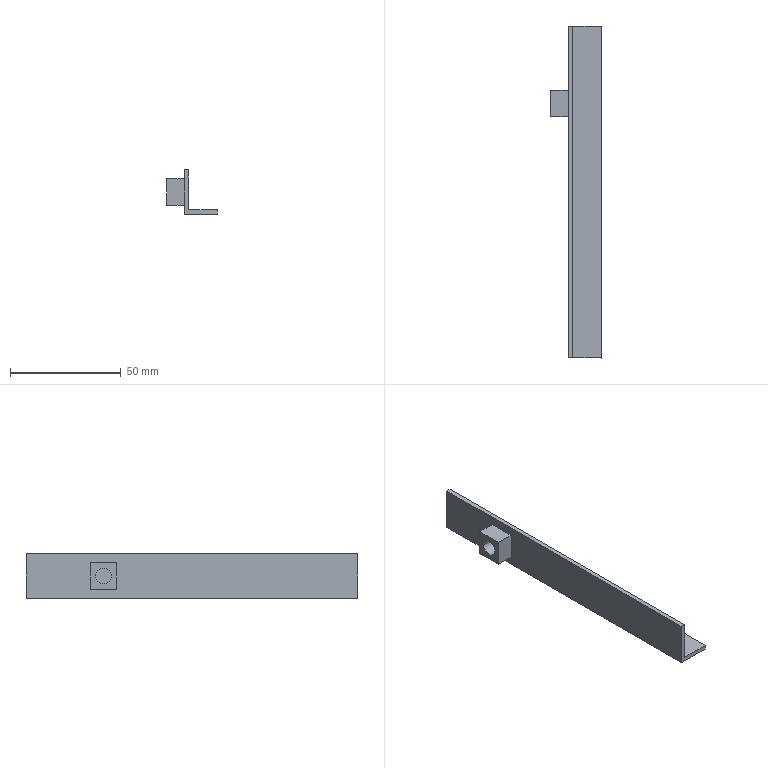Part | SolidWorks | features ICE 2, Cut 1, Extrusion 1 | 1 solid | 16 faces | box 23 x 150 x 20 mm | volume 10744 mm3 | plane 14 | cylinder 2 | commonest cylinder face diameters 7 x2
STEP:
#1=CARTESIAN_POINT('',(84.5,-3.5,10.));
#2=VERTEX_POINT('',#1);
#3=CARTESIAN_POINT('',(84.5,3.5,10.));
#4=VERTEX_POINT('',#3);
#5=CARTESIAN_POINT('',(84.5,0.,10.));
#6=DIRECTION('',(1.,0.,0.));
#7=DIRECTION('',(0.,1.,0.));
#8=AXIS2_PLACEMENT_3D('',#5,#6,#7);
#9=CIRCLE('',#8,3.5);
#10=EDGE_CURVE('',#2,#4,#9,.T.);
#11=ORIENTED_EDGE('',*,*,#10,.F.);
#12=CARTESIAN_POINT('',(92.5,-3.5,10.));
#13=VERTEX_POINT('',#12);
#14=CARTESIAN_POINT('',(84.5,-3.5,10.));
#15=DIRECTION('',(1.,0.,0.));
#16=VECTOR('',#15,1000.);
#17=LINE('',#14,#16);
#18=EDGE_CURVE('',#2,#13,#17,.T.);
#19=ORIENTED_EDGE('',*,*,#18,.T.);
#20=CARTESIAN_POINT('',(92.5,3.5,10.));
#21=VERTEX_POINT('',#20);
#22=CARTESIAN_POINT('',(92.5,0.,10.));
#23=DIRECTION('',(1.,0.,0.));
#24=DIRECTION('',(0.,1.,0.));
#25=AXIS2_PLACEMENT_3D('',#22,#23,#24);
#26=CIRCLE('',#25,3.5);
#27=EDGE_CURVE('',#13,#21,#26,.T.);
#28=ORIENTED_EDGE('',*,*,#27,.T.);
#29=CARTESIAN_POINT('',(84.5,3.5,10.));
#30=DIRECTION('',(1.,0.,0.));
#31=VECTOR('',#30,1000.);
#32=LINE('',#29,#31);
#33=EDGE_CURVE('',#4,#21,#32,.T.);
#34=ORIENTED_EDGE('',*,*,#33,.F.);
#35=EDGE_LOOP('',(#11,#19,#28,#34));
#36=FACE_OUTER_BOUND('',#35,.T.);
#37=CARTESIAN_POINT('',(84.5,0.,10.));
#38=DIRECTION('',(1.,0.,0.));
#39=DIRECTION('',(0.,1.,0.));
#40=AXIS2_PLACEMENT_3D('',#37,#38,#39);
#41=CYLINDRICAL_SURFACE('',#40,3.5);
#42=ADVANCED_FACE('',(#36),#41,.F.);
#43=CARTESIAN_POINT('',(92.5,6.,4.));
#44=VERTEX_POINT('',#43);
#45=CARTESIAN_POINT('',(92.5,6.,16.));
#46=VERTEX_POINT('',#45);
#47=CARTESIAN_POINT('',(92.5,6.,20.));
#48=DIRECTION('',(0.,0.,1.));
#49=VECTOR('',#48,1000.);
#50=LINE('',#47,#49);
#51=EDGE_CURVE('',#44,#46,#50,.T.);
#52=ORIENTED_EDGE('',*,*,#51,.T.);
#53=CARTESIAN_POINT('',(92.5,-6.,16.));
#54=VERTEX_POINT('',#53);
#55=CARTESIAN_POINT('',(92.5,35.,16.));
#56=DIRECTION('',(0.,-1.,0.));
#57=VECTOR('',#56,1000.);
#58=LINE('',#55,#57);
#59=EDGE_CURVE('',#46,#54,#58,.T.);
#60=ORIENTED_EDGE('',*,*,#59,.T.);
#61=CARTESIAN_POINT('',(92.5,-6.,4.));
#62=VERTEX_POINT('',#61);
#63=CARTESIAN_POINT('',(92.5,-6.,20.));
#64=DIRECTION('',(0.,0.,-1.));
#65=VECTOR('',#64,1000.);
#66=LINE('',#63,#65);
#67=EDGE_CURVE('',#54,#62,#66,.T.);
#68=ORIENTED_EDGE('',*,*,#67,.T.);
#69=CARTESIAN_POINT('',(92.5,35.,4.));
#70=DIRECTION('',(0.,1.,0.));
#71=VECTOR('',#70,1000.);
#72=LINE('',#69,#71);
#73=EDGE_CURVE('',#62,#44,#72,.T.);
#74=ORIENTED_EDGE('',*,*,#73,.T.);
#75=EDGE_LOOP('',(#52,#60,#68,#74));
#76=FACE_BOUND('',#75,.T.);
#77=CARTESIAN_POINT('',(92.5,35.,0.));
#78=VERTEX_POINT('',#77);
#79=CARTESIAN_POINT('',(92.5,-115.,0.));
#80=VERTEX_POINT('',#79);
#81=CARTESIAN_POINT('',(92.5,35.,0.));
#82=DIRECTION('',(0.,-1.,0.));
#83=VECTOR('',#82,1000.);
#84=LINE('',#81,#83);
#85=EDGE_CURVE('',#78,#80,#84,.T.);
#86=ORIENTED_EDGE('',*,*,#85,.T.);
#87=CARTESIAN_POINT('',(92.5,-115.,20.));
#88=VERTEX_POINT('',#87);
#89=CARTESIAN_POINT('',(92.5,-115.,20.));
#90=DIRECTION('',(0.,0.,-1.));
#91=VECTOR('',#90,1000.);
#92=LINE('',#89,#91);
#93=EDGE_CURVE('',#88,#80,#92,.T.);
#94=ORIENTED_EDGE('',*,*,#93,.F.);
#95=CARTESIAN_POINT('',(92.5,35.,20.));
#96=VERTEX_POINT('',#95);
#97=CARTESIAN_POINT('',(92.5,35.,20.));
#98=DIRECTION('',(0.,-1.,0.));
#99=VECTOR('',#98,1000.);
#100=LINE('',#97,#99);
#101=EDGE_CURVE('',#96,#88,#100,.T.);
#102=ORIENTED_EDGE('',*,*,#101,.F.);
#103=CARTESIAN_POINT('',(92.5,35.,20.));
#104=DIRECTION('',(0.,0.,-1.));
#105=VECTOR('',#104,1000.);
#106=LINE('',#103,#105);
#107=EDGE_CURVE('',#96,#78,#106,.T.);
#108=ORIENTED_EDGE('',*,*,#107,.T.);
#109=EDGE_LOOP('',(#86,#94,#102,#108));
#110=FACE_OUTER_BOUND('',#109,.T.);
#111=CARTESIAN_POINT('',(92.5,35.,20.));
#112=DIRECTION('',(1.,0.,0.));
#113=DIRECTION('',(0.,1.,0.));
#114=AXIS2_PLACEMENT_3D('',#111,#112,#113);
#115=PLANE('',#114);
#116=ADVANCED_FACE('',(#76,#110),#115,.F.);
#117=CARTESIAN_POINT('',(107.5,35.,2.));
#118=VERTEX_POINT('',#117);
#119=CARTESIAN_POINT('',(107.5,35.,0.));
#120=VERTEX_POINT('',#119);
#121=CARTESIAN_POINT('',(107.5,35.,20.));
#122=DIRECTION('',(0.,0.,-1.));
#123=VECTOR('',#122,1000.);
#124=LINE('',#121,#123);
#125=EDGE_CURVE('',#118,#120,#124,.T.);
#126=ORIENTED_EDGE('',*,*,#125,.F.);
#127=CARTESIAN_POINT('',(107.5,-115.,2.));
#128=VERTEX_POINT('',#127);
#129=CARTESIAN_POINT('',(107.5,119.,2.));
#130=DIRECTION('',(0.,-1.,0.));
#131=VECTOR('',#130,1000.);
#132=LINE('',#129,#131);
#133=EDGE_CURVE('',#118,#128,#132,.T.);
#134=ORIENTED_EDGE('',*,*,#133,.T.);
#135=CARTESIAN_POINT('',(107.5,-115.,0.));
#136=VERTEX_POINT('',#135);
#137=CARTESIAN_POINT('',(107.5,-115.,0.));
#138=DIRECTION('',(0.,0.,1.));
#139=VECTOR('',#138,1000.);
#140=LINE('',#137,#139);
#141=EDGE_CURVE('',#136,#128,#140,.T.);
#142=ORIENTED_EDGE('',*,*,#141,.F.);
#143=CARTESIAN_POINT('',(107.5,35.,0.));
#144=DIRECTION('',(0.,1.,0.));
#145=VECTOR('',#144,1000.);
#146=LINE('',#143,#145);
#147=EDGE_CURVE('',#136,#120,#146,.T.);
#148=ORIENTED_EDGE('',*,*,#147,.T.);
#149=EDGE_LOOP('',(#126,#134,#142,#148));
#150=FACE_OUTER_BOUND('',#149,.T.);
#151=CARTESIAN_POINT('',(107.5,35.,20.));
#152=DIRECTION('',(-1.,0.,0.));
#153=DIRECTION('',(0.,0.,1.));
#154=AXIS2_PLACEMENT_3D('',#151,#152,#153);
#155=PLANE('',#154);
#156=ADVANCED_FACE('',(#150),#155,.F.);
#157=CARTESIAN_POINT('',(94.5,35.,20.));
#158=VERTEX_POINT('',#157);
#159=CARTESIAN_POINT('',(94.5,35.,2.));
#160=VERTEX_POINT('',#159);
#161=CARTESIAN_POINT('',(94.5,35.,20.));
#162=DIRECTION('',(0.,0.,-1.));
#163=VECTOR('',#162,1000.);
#164=LINE('',#161,#163);
#165=EDGE_CURVE('',#158,#160,#164,.T.);
#166=ORIENTED_EDGE('',*,*,#165,.T.);
#167=CARTESIAN_POINT('',(107.5,35.,2.));
#168=DIRECTION('',(1.,0.,0.));
#169=VECTOR('',#168,1000.);
#170=LINE('',#167,#169);
#171=EDGE_CURVE('',#160,#118,#170,.T.);
#172=ORIENTED_EDGE('',*,*,#171,.T.);
#173=ORIENTED_EDGE('',*,*,#125,.T.);
#174=CARTESIAN_POINT('',(107.5,35.,0.));
#175=DIRECTION('',(-1.,0.,0.));
#176=VECTOR('',#175,1000.);
#177=LINE('',#174,#176);
#178=EDGE_CURVE('',#120,#78,#177,.T.);
#179=ORIENTED_EDGE('',*,*,#178,.T.);
#180=ORIENTED_EDGE('',*,*,#107,.F.);
#181=CARTESIAN_POINT('',(107.5,35.,20.));
#182=DIRECTION('',(-1.,0.,0.));
#183=VECTOR('',#182,1000.);
#184=LINE('',#181,#183);
#185=EDGE_CURVE('',#158,#96,#184,.T.);
#186=ORIENTED_EDGE('',*,*,#185,.F.);
#187=EDGE_LOOP('',(#166,#172,#173,#179,#180,#186));
#188=FACE_OUTER_BOUND('',#187,.T.);
#189=CARTESIAN_POINT('',(107.5,35.,20.));
#190=DIRECTION('',(0.,-1.,0.));
#191=DIRECTION('',(1.,0.,0.));
#192=AXIS2_PLACEMENT_3D('',#189,#190,#191);
#193=PLANE('',#192);
#194=ADVANCED_FACE('',(#188),#193,.F.);
#195=ORIENTED_EDGE('',*,*,#101,.T.);
#196=CARTESIAN_POINT('',(94.5,-115.,20.));
#197=VERTEX_POINT('',#196);
#198=CARTESIAN_POINT('',(94.5,-115.,20.));
#199=DIRECTION('',(-1.,0.,0.));
#200=VECTOR('',#199,1000.);
#201=LINE('',#198,#200);
#202=EDGE_CURVE('',#197,#88,#201,.T.);
#203=ORIENTED_EDGE('',*,*,#202,.F.);
#204=CARTESIAN_POINT('',(94.5,0.,20.));
#205=DIRECTION('',(0.,1.,0.));
#206=VECTOR('',#205,1000.);
#207=LINE('',#204,#206);
#208=EDGE_CURVE('',#197,#158,#207,.T.);
#209=ORIENTED_EDGE('',*,*,#208,.T.);
#210=ORIENTED_EDGE('',*,*,#185,.T.);
#211=EDGE_LOOP('',(#195,#203,#209,#210));
#212=FACE_OUTER_BOUND('',#211,.T.);
#213=CARTESIAN_POINT('',(0.,0.,20.));
#214=DIRECTION('',(0.,0.,-1.));
#215=DIRECTION('',(-1.,0.,0.));
#216=AXIS2_PLACEMENT_3D('',#213,#214,#215);
#217=PLANE('',#216);
#218=ADVANCED_FACE('',(#212),#217,.F.);
#219=ORIENTED_EDGE('',*,*,#85,.F.);
#220=ORIENTED_EDGE('',*,*,#178,.F.);
#221=ORIENTED_EDGE('',*,*,#147,.F.);
#222=CARTESIAN_POINT('',(92.5,-115.,0.));
#223=DIRECTION('',(1.,0.,0.));
#224=VECTOR('',#223,1000.);
#225=LINE('',#222,#224);
#226=EDGE_CURVE('',#80,#136,#225,.T.);
#227=ORIENTED_EDGE('',*,*,#226,.F.);
#228=EDGE_LOOP('',(#219,#220,#221,#227));
#229=FACE_OUTER_BOUND('',#228,.T.);
#230=CARTESIAN_POINT('',(0.,0.,0.));
#231=DIRECTION('',(0.,0.,-1.));
#232=DIRECTION('',(-1.,0.,0.));
#233=AXIS2_PLACEMENT_3D('',#230,#231,#232);
#234=PLANE('',#233);
#235=ADVANCED_FACE('',(#229),#234,.T.);
#236=CARTESIAN_POINT('',(94.5,-115.,2.));
#237=VERTEX_POINT('',#236);
#238=CARTESIAN_POINT('',(94.5,119.,2.));
#239=DIRECTION('',(0.,-1.,0.));
#240=VECTOR('',#239,1000.);
#241=LINE('',#238,#240);
#242=EDGE_CURVE('',#160,#237,#241,.T.);
#243=ORIENTED_EDGE('',*,*,#242,.T.);
#244=CARTESIAN_POINT('',(107.5,-115.,2.));
#245=DIRECTION('',(-1.,0.,0.));
#246=VECTOR('',#245,1000.);
#247=LINE('',#244,#246);
#248=EDGE_CURVE('',#128,#237,#247,.T.);
#249=ORIENTED_EDGE('',*,*,#248,.F.);
#250=ORIENTED_EDGE('',*,*,#133,.F.);
#251=ORIENTED_EDGE('',*,*,#171,.F.);
#252=EDGE_LOOP('',(#243,#249,#250,#251));
#253=FACE_OUTER_BOUND('',#252,.T.);
#254=CARTESIAN_POINT('',(107.5,119.,2.));
#255=DIRECTION('',(0.,0.,-1.));
#256=DIRECTION('',(-1.,0.,0.));
#257=AXIS2_PLACEMENT_3D('',#254,#255,#256);
#258=PLANE('',#257);
#259=ADVANCED_FACE('',(#253),#258,.F.);
#260=ORIENTED_EDGE('',*,*,#208,.F.);
#261=CARTESIAN_POINT('',(94.5,-115.,2.));
#262=DIRECTION('',(0.,0.,1.));
#263=VECTOR('',#262,1000.);
#264=LINE('',#261,#263);
#265=EDGE_CURVE('',#237,#197,#264,.T.);
#266=ORIENTED_EDGE('',*,*,#265,.F.);
#267=ORIENTED_EDGE('',*,*,#242,.F.);
#268=ORIENTED_EDGE('',*,*,#165,.F.);
#269=EDGE_LOOP('',(#260,#266,#267,#268));
#270=FACE_OUTER_BOUND('',#269,.T.);
#271=CARTESIAN_POINT('',(94.5,119.,2.));
#272=DIRECTION('',(-1.,0.,0.));
#273=DIRECTION('',(0.,-1.,0.));
#274=AXIS2_PLACEMENT_3D('',#271,#272,#273);
#275=PLANE('',#274);
#276=ADVANCED_FACE('',(#270),#275,.F.);
#277=ORIENTED_EDGE('',*,*,#226,.T.);
#278=ORIENTED_EDGE('',*,*,#141,.T.);
#279=ORIENTED_EDGE('',*,*,#248,.T.);
#280=ORIENTED_EDGE('',*,*,#265,.T.);
#281=ORIENTED_EDGE('',*,*,#202,.T.);
#282=ORIENTED_EDGE('',*,*,#93,.T.);
#283=EDGE_LOOP('',(#277,#278,#279,#280,#281,#282));
#284=FACE_OUTER_BOUND('',#283,.T.);
#285=CARTESIAN_POINT('',(0.,-115.,0.));
#286=DIRECTION('',(0.,-1.,0.));
#287=DIRECTION('',(1.,0.,0.));
#288=AXIS2_PLACEMENT_3D('',#285,#286,#287);
#289=PLANE('',#288);
#290=ADVANCED_FACE('',(#284),#289,.T.);
#291=ORIENTED_EDGE('',*,*,#59,.F.);
#292=CARTESIAN_POINT('',(84.5,6.,16.));
#293=VERTEX_POINT('',#292);
#294=CARTESIAN_POINT('',(84.5,6.,16.));
#295=DIRECTION('',(1.,0.,0.));
#296=VECTOR('',#295,1000.);
#297=LINE('',#294,#296);
#298=EDGE_CURVE('',#293,#46,#297,.T.);
#299=ORIENTED_EDGE('',*,*,#298,.F.);
#300=CARTESIAN_POINT('',(84.5,-6.,16.));
#301=VERTEX_POINT('',#300);
#302=CARTESIAN_POINT('',(84.5,-6.,16.));
#303=DIRECTION('',(0.,-1.,0.));
#304=VECTOR('',#303,1000.);
#305=LINE('',#302,#304);
#306=EDGE_CURVE('',#293,#301,#305,.T.);
#307=ORIENTED_EDGE('',*,*,#306,.T.);
#308=CARTESIAN_POINT('',(84.5,-6.,16.));
#309=DIRECTION('',(1.,0.,0.));
#310=VECTOR('',#309,1000.);
#311=LINE('',#308,#310);
#312=EDGE_CURVE('',#301,#54,#311,.T.);
#313=ORIENTED_EDGE('',*,*,#312,.T.);
#314=EDGE_LOOP('',(#291,#299,#307,#313));
#315=FACE_OUTER_BOUND('',#314,.T.);
#316=CARTESIAN_POINT('',(84.5,-6.,16.));
#317=DIRECTION('',(0.,0.,1.));
#318=DIRECTION('',(1.,0.,0.));
#319=AXIS2_PLACEMENT_3D('',#316,#317,#318);
#320=PLANE('',#319);
#321=ADVANCED_FACE('',(#315),#320,.T.);
#322=ORIENTED_EDGE('',*,*,#51,.F.);
#323=CARTESIAN_POINT('',(84.5,6.,4.));
#324=VERTEX_POINT('',#323);
#325=CARTESIAN_POINT('',(84.5,6.,4.));
#326=DIRECTION('',(1.,0.,0.));
#327=VECTOR('',#326,1000.);
#328=LINE('',#325,#327);
#329=EDGE_CURVE('',#324,#44,#328,.T.);
#330=ORIENTED_EDGE('',*,*,#329,.F.);
#331=CARTESIAN_POINT('',(84.5,6.,4.));
#332=DIRECTION('',(0.,0.,1.));
#333=VECTOR('',#332,1000.);
#334=LINE('',#331,#333);
#335=EDGE_CURVE('',#324,#293,#334,.T.);
#336=ORIENTED_EDGE('',*,*,#335,.T.);
#337=ORIENTED_EDGE('',*,*,#298,.T.);
#338=EDGE_LOOP('',(#322,#330,#336,#337));
#339=FACE_OUTER_BOUND('',#338,.T.);
#340=CARTESIAN_POINT('',(84.5,6.,4.));
#341=DIRECTION('',(0.,1.,0.));
#342=DIRECTION('',(-1.,0.,0.));
#343=AXIS2_PLACEMENT_3D('',#340,#341,#342);
#344=PLANE('',#343);
#345=ADVANCED_FACE('',(#339),#344,.T.);
#346=ORIENTED_EDGE('',*,*,#73,.F.);
#347=CARTESIAN_POINT('',(84.5,-6.,4.));
#348=VERTEX_POINT('',#347);
#349=CARTESIAN_POINT('',(84.5,-6.,4.));
#350=DIRECTION('',(1.,0.,0.));
#351=VECTOR('',#350,1000.);
#352=LINE('',#349,#351);
#353=EDGE_CURVE('',#348,#62,#352,.T.);
#354=ORIENTED_EDGE('',*,*,#353,.F.);
#355=CARTESIAN_POINT('',(84.5,-6.,4.));
#356=DIRECTION('',(0.,1.,0.));
#357=VECTOR('',#356,1000.);
#358=LINE('',#355,#357);
#359=EDGE_CURVE('',#348,#324,#358,.T.);
#360=ORIENTED_EDGE('',*,*,#359,.T.);
#361=ORIENTED_EDGE('',*,*,#329,.T.);
#362=EDGE_LOOP('',(#346,#354,#360,#361));
#363=FACE_OUTER_BOUND('',#362,.T.);
#364=CARTESIAN_POINT('',(84.5,-6.,4.));
#365=DIRECTION('',(0.,0.,-1.));
#366=DIRECTION('',(-1.,0.,0.));
#367=AXIS2_PLACEMENT_3D('',#364,#365,#366);
#368=PLANE('',#367);
#369=ADVANCED_FACE('',(#363),#368,.T.);
#370=ORIENTED_EDGE('',*,*,#67,.F.);
#371=ORIENTED_EDGE('',*,*,#312,.F.);
#372=CARTESIAN_POINT('',(84.5,-6.,4.));
#373=DIRECTION('',(0.,0.,-1.));
#374=VECTOR('',#373,1000.);
#375=LINE('',#372,#374);
#376=EDGE_CURVE('',#301,#348,#375,.T.);
#377=ORIENTED_EDGE('',*,*,#376,.T.);
#378=ORIENTED_EDGE('',*,*,#353,.T.);
#379=EDGE_LOOP('',(#370,#371,#377,#378));
#380=FACE_OUTER_BOUND('',#379,.T.);
#381=CARTESIAN_POINT('',(84.5,-6.,4.));
#382=DIRECTION('',(0.,-1.,0.));
#383=DIRECTION('',(1.,0.,0.));
#384=AXIS2_PLACEMENT_3D('',#381,#382,#383);
#385=PLANE('',#384);
#386=ADVANCED_FACE('',(#380),#385,.T.);
#387=ORIENTED_EDGE('',*,*,#18,.F.);
#388=CARTESIAN_POINT('',(84.5,0.,10.));
#389=DIRECTION('',(1.,0.,0.));
#390=DIRECTION('',(0.,1.,0.));
#391=AXIS2_PLACEMENT_3D('',#388,#389,#390);
#392=CIRCLE('',#391,3.5);
#393=EDGE_CURVE('',#4,#2,#392,.T.);
#394=ORIENTED_EDGE('',*,*,#393,.F.);
#395=ORIENTED_EDGE('',*,*,#33,.T.);
#396=CARTESIAN_POINT('',(92.5,0.,10.));
#397=DIRECTION('',(1.,0.,0.));
#398=DIRECTION('',(0.,1.,0.));
#399=AXIS2_PLACEMENT_3D('',#396,#397,#398);
#400=CIRCLE('',#399,3.5);
#401=EDGE_CURVE('',#21,#13,#400,.T.);
#402=ORIENTED_EDGE('',*,*,#401,.T.);
#403=EDGE_LOOP('',(#387,#394,#395,#402));
#404=FACE_OUTER_BOUND('',#403,.T.);
#405=CARTESIAN_POINT('',(84.5,0.,10.));
#406=DIRECTION('',(1.,0.,0.));
#407=DIRECTION('',(0.,1.,0.));
#408=AXIS2_PLACEMENT_3D('',#405,#406,#407);
#409=CYLINDRICAL_SURFACE('',#408,3.5);
#410=ADVANCED_FACE('',(#404),#409,.F.);
#411=ORIENTED_EDGE('',*,*,#393,.T.);
#412=ORIENTED_EDGE('',*,*,#10,.T.);
#413=EDGE_LOOP('',(#411,#412));
#414=FACE_BOUND('',#413,.T.);
#415=ORIENTED_EDGE('',*,*,#306,.F.);
#416=ORIENTED_EDGE('',*,*,#335,.F.);
#417=ORIENTED_EDGE('',*,*,#359,.F.);
#418=ORIENTED_EDGE('',*,*,#376,.F.);
#419=EDGE_LOOP('',(#415,#416,#417,#418));
#420=FACE_OUTER_BOUND('',#419,.T.);
#421=CARTESIAN_POINT('',(84.5,0.,0.));
#422=DIRECTION('',(1.,0.,0.));
#423=DIRECTION('',(0.,0.,-1.));
#424=AXIS2_PLACEMENT_3D('',#421,#422,#423);
#425=PLANE('',#424);
#426=ADVANCED_FACE('',(#414,#420),#425,.F.);
#427=ORIENTED_EDGE('',*,*,#401,.F.);
#428=ORIENTED_EDGE('',*,*,#27,.F.);
#429=EDGE_LOOP('',(#427,#428));
#430=FACE_OUTER_BOUND('',#429,.T.);
#431=CARTESIAN_POINT('',(92.5,35.,20.));
#432=DIRECTION('',(1.,0.,0.));
#433=DIRECTION('',(0.,1.,0.));
#434=AXIS2_PLACEMENT_3D('',#431,#432,#433);
#435=PLANE('',#434);
#436=ADVANCED_FACE('',(#430),#435,.F.);
#437=CLOSED_SHELL('',(#42,#116,#156,#194,#218,#235,#259,#276,#290,#321,#345,#369,#386,#410,#426,#436));
#438=MANIFOLD_SOLID_BREP('',#437);
#439=CARTESIAN_POINT('',(0.,0.,0.));
#440=DIRECTION('',(0.,0.,1.));
#441=DIRECTION('',(1.,0.,0.));
#442=AXIS2_PLACEMENT_3D('',#439,#440,#441);
#443=(LENGTH_UNIT()NAMED_UNIT(*)SI_UNIT(.MILLI.,.METRE.));
#444=UNCERTAINTY_MEASURE_WITH_UNIT(LENGTH_MEASURE(0.00001),#443,'','');
#445=(NAMED_UNIT(*)PLANE_ANGLE_UNIT()SI_UNIT($,.RADIAN.));
#446=(NAMED_UNIT(*)SI_UNIT($,.STERADIAN.)SOLID_ANGLE_UNIT());
#447=(GEOMETRIC_REPRESENTATION_CONTEXT(3)GLOBAL_UNCERTAINTY_ASSIGNED_CONTEXT((#444))GLOBAL_UNIT_ASSIGNED_CONTEXT((#443,#445,#446))REPRESENTATION_CONTEXT('',''));
#448=ADVANCED_BREP_SHAPE_REPRESENTATION('',(#438,#442),#447);